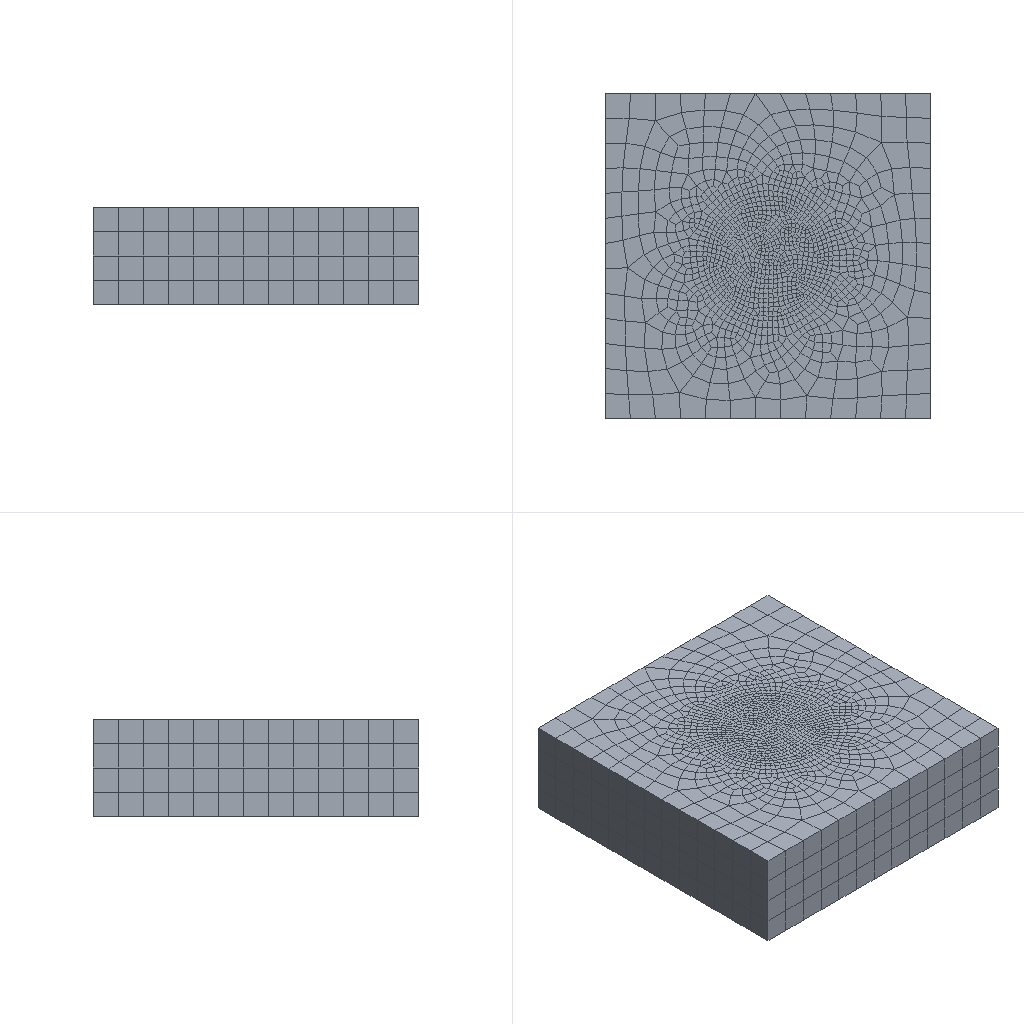Simulation study | abaqus
Set-up summary:
category,name,step,type,value,unit,region
solver,abaqus
solver,version,,,Abaqus/Explicit 2020
units,not stated in the deck,,not stated
analysis,deck,,transient,transient
load_step,Step-1,Step-1,transient,nlgeom=True
contact,interactions,,,general=1 pairs=1 ties=0
load_step,requested,,,1
mesh,nodes,,,8749
mesh,elements,,,7211
element_type,R3D3,,rigid,22
element_type,R3D4,,rigid,1545
element_type,C3D8R,,solid,5644
load,load commands in deck,,count,2
bc,support commands in deck,,count,7
material,WORK,,in results
check,setup vs results,,match,"per instance, exact: element labels, types and connectivity; labels of the nodes the elements use; coordinates of those nodes at SINGLE_PRECISION in 2 of 2 instance(s)"
Abaqus input file, long lists of numbers shortened:
*Heading
** Job name: Job-3 Model name: Model-1-Copy-Copy
** Generated by: Abaqus/CAE 2020
*Preprint, echo=NO, model=NO, history=NO, contact=NO
**
** PARTS
**
*Part, name=tool
*Node
      1,  0.7192,   1.154,  0.8171
      2,   2.821,   1.02,   1.803
** (1556 more lines like these left out)
*Element, type=R3D4
  1,   1,  28, 320,  67
  2,  28,  29, 321, 320
** (1543 more lines like these left out)
*Element, type=R3D3
1041, 1227, 1197, 1198
1042,   48,    3,  110
** (20 more lines like these left out)
*Node
   1559, 3.33066907e-16, 1.77635684e-15,           6.
*Nset, nset=tool-RefPt_, internal
1559,
*Elset, elset=tool, generate
    1,  1567,     1
*End Part
**
*Part, name=work
*Node
      1,         3.75,         -40.,           0.
      2,        23.75,         -40.,           0.
** (7188 more lines like these left out)
*Element, type=C3D8R
   1,  373,  319,  323,  418, 3373, 3319, 3323, 3418
   2,  111,  112,  301,  311, 1686, 1687, 3301, 3311
** (5642 more lines like these left out)
*Nset, nset=Set-7, generate
    1,  7190,     1
*Elset, elset=Set-7, generate
    1,  5644,     1
** Section: wok
*Solid Section, elset=Set-7, material=work
,
*End Part
**
**
** ASSEMBLY
**
*Assembly, name=Assembly
**
*Instance, name=tool-1, part=tool
          0.,           0.,           0.
          0.,           0.,           0.,           0.,           0., -1., 25.
*End Instance
**
*Instance, name=work-1, part=work
      -13.75,          50.,          -6.
*End Instance
**
*Nset, nset=Set-1, instance=tool-1
 1559,
*Nset, nset=Set-5, instance=work-1
    1,    2,    3,    4,    6,    7,    8,    9,   11,   12,   13,   14,   15,   16,   17,   18
   19,   20,   21,   22,   23,   24,   25,   26,   27,   28,   29,   30,   31,   32,   33,   34
** (15 more lines like these left out)
*Elset, elset=Set-5, instance=work-1
   24,   25,   35,   47,   48,   59,  514,  518,  533,  534,  561,  565,  567,  570,  571,  582
  583,  588,  589,  591,  593,  595,  597,  598,  599,  607,  608,  610,  612,  613,  618,  620
** (10 more lines like these left out)
*Nset, nset=Set-6, instance=tool-1
 1559,
*Nset, nset=s_Set-4, instance=work-1
    5,   10,   59,   60,   61,   62,   63,   64,   65,   66,   67,   68,   69,   70,   71,   72
   73,   74,   75,   76,   77,   78,   79,   80,   81,   82,   83,   84,   85,   86,   87,   88
** (243 more lines like these left out)
*Elset, elset=s_Set-4, instance=work-1, generate
 2681,  5644,     1
*Elset, elset=_m_Surf-1_SPOS, internal, instance=tool-1, generate
    1,  1567,     1
*Surface, type=ELEMENT, name=m_Surf-1
_m_Surf-1_SPOS, SPOS
*Surface, type=NODE, name=s_Set-4_CNS_, internal
s_Set-4, 1.
*Rigid Body, ref node=tool-1.tool-RefPt_, elset=tool-1.tool
*End Assembly
*Amplitude, name=Amp-1
             0.,              0.,           0.001,              1.
*Amplitude, name=Amp-2
             0.,              0.,            0.01,              1.
**
** MATERIALS
**
*Material, name=work
*Damage Initiation, criterion=JOHNSON COOK
 0.13,  0.13,  -1.5, 0.011,    0.,  600.,   25.,    1.
*Damage Evolution, type=DISPLACEMENT
 0.05,
*Density
 2.77e-09,
*Elastic
71700., 0.33
*Plastic, hardening=JOHNSON COOK
369., 684., 0.73,  1.7, 600.,  25.
*Rate Dependent, type=JOHNSON COOK
 0.0083,1.
**
** INTERACTION PROPERTIES
**
*Surface Interaction, name=IntProp-1
*Friction
 0.15,
*Surface Behavior, pressure-overclosure=HARD
** ----------------------------------------------------------------
**
** STEP: Step-1
**
*Step, name=Step-1, nlgeom=YES
*Dynamic, Explicit
, 0.1
*Bulk Viscosity
0.06, 1.2
** Mass Scaling: Semi-Automatic
**               Whole Model
*Fixed Mass Scaling, factor=500.
**
** BOUNDARY CONDITIONS
**
** Name: BC-2 Type: 对称/反对称/完全固定
*Boundary
Set-5, ENCASTRE
** Name: BC-3 Type: 速度/角速度
*Boundary, type=VELOCITY
Set-6, 1, 1
Set-6, 2, 2
Set-6, 3, 3, -60.
Set-6, 4, 4
Set-6, 5, 5
Set-6, 6, 6, -60.
**
** INTERACTIONS
**
** Interaction: Int-1
*Contact Pair, interaction=IntProp-1, mechanical constraint=KINEMATIC, cpset=Int-1
m_Surf-1, s_Set-4_CNS_
** Interaction: Int-3
*Contact, op=NEW
*Contact Inclusions, ALL EXTERIOR
*Contact Property Assignment
 ,  , IntProp-1
**
** OUTPUT REQUESTS
**
*Restart, write, number interval=1, time marks=NO
**
** FIELD OUTPUT: F-Output-1
**
*Output, field, number interval=100
*Node Output
A, RF, U, V
*Element Output, directions=YES
E, EVF, LE, MISES, MISESMAX, PE, PEEQ, PEEQMAX, PEEQT, PEEQVAVG, PEMAG, PEVAVG, PRESSONLY, S, SEQUT, STATUS
SVAVG, YIELDPOT
*Contact Output
CSTRESS,
**
** HISTORY OUTPUT: H-Output-1
**
*Output, history, variable=PRESELECT
*End Step
Results summary:
result,step,Step-1,completed,increments=162966 time=0.1/0.1
result,analysis,,,transient
result,last_loadstep,,,1
result,analysis steps,,count,1
result,primary field,,,U
result,reaction total,,FX,-71.578,model units
result,reaction total,,FY,135.266,model units
result,reaction total,,FZ,326.798,model units